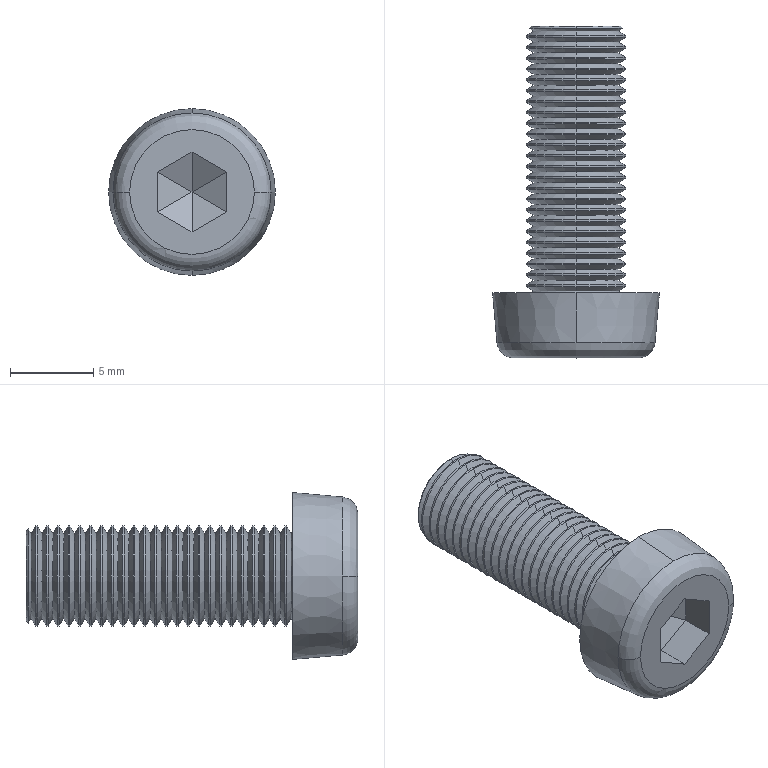Part | SolidWorks | features BaseBody 1 | 1 solid | 172 faces | box 10 x 19.9 x 10 mm | volume 638.621 mm3 | cone 104 | cylinder 50 | plane 16 | torus 2 | commonest cylinder face diameters 6 x48 7.083 x2